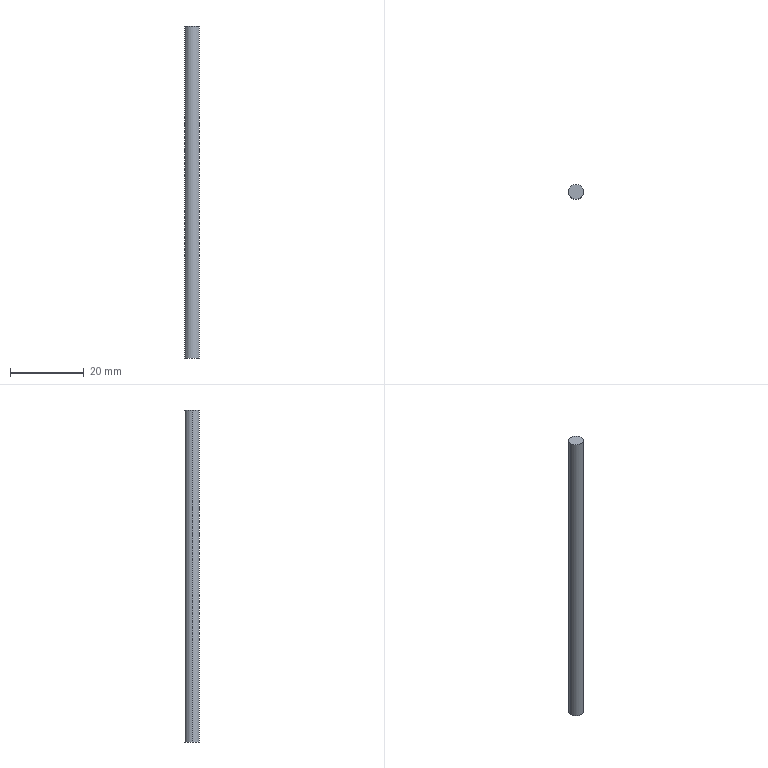Part | SolidWorks | features Extrusion 1 | 1 solid | 4 faces | box 4 x 4 x 90 mm | volume 1131 mm3 | cylinder 2 | plane 2 | commonest cylinder face diameters 4 x2
STEP:
#1=CARTESIAN_POINT('',(2.,0.,90.));
#2=VERTEX_POINT('',#1);
#3=CARTESIAN_POINT('',(-2.,0.,90.));
#4=VERTEX_POINT('',#3);
#5=CARTESIAN_POINT('',(0.,0.,90.));
#6=DIRECTION('',(0.,0.,1.));
#7=DIRECTION('',(1.,0.,0.));
#8=AXIS2_PLACEMENT_3D('',#5,#6,#7);
#9=CIRCLE('',#8,2.);
#10=EDGE_CURVE('',#2,#4,#9,.T.);
#11=ORIENTED_EDGE('',*,*,#10,.F.);
#12=CARTESIAN_POINT('',(2.,0.,0.));
#13=VERTEX_POINT('',#12);
#14=CARTESIAN_POINT('',(2.,0.,90.));
#15=DIRECTION('',(0.,0.,-1.));
#16=VECTOR('',#15,1000.);
#17=LINE('',#14,#16);
#18=EDGE_CURVE('',#2,#13,#17,.T.);
#19=ORIENTED_EDGE('',*,*,#18,.T.);
#20=CARTESIAN_POINT('',(-2.,0.,0.));
#21=VERTEX_POINT('',#20);
#22=CARTESIAN_POINT('',(0.,0.,0.));
#23=DIRECTION('',(0.,0.,1.));
#24=DIRECTION('',(1.,0.,0.));
#25=AXIS2_PLACEMENT_3D('',#22,#23,#24);
#26=CIRCLE('',#25,2.);
#27=EDGE_CURVE('',#13,#21,#26,.T.);
#28=ORIENTED_EDGE('',*,*,#27,.T.);
#29=CARTESIAN_POINT('',(-2.,0.,90.));
#30=DIRECTION('',(0.,0.,-1.));
#31=VECTOR('',#30,1000.);
#32=LINE('',#29,#31);
#33=EDGE_CURVE('',#4,#21,#32,.T.);
#34=ORIENTED_EDGE('',*,*,#33,.F.);
#35=EDGE_LOOP('',(#11,#19,#28,#34));
#36=FACE_OUTER_BOUND('',#35,.T.);
#37=CARTESIAN_POINT('',(0.,0.,90.));
#38=DIRECTION('',(0.,0.,-1.));
#39=DIRECTION('',(-1.,0.,0.));
#40=AXIS2_PLACEMENT_3D('',#37,#38,#39);
#41=CYLINDRICAL_SURFACE('',#40,2.);
#42=ADVANCED_FACE('',(#36),#41,.T.);
#43=ORIENTED_EDGE('',*,*,#18,.F.);
#44=CARTESIAN_POINT('',(0.,0.,90.));
#45=DIRECTION('',(0.,0.,1.));
#46=DIRECTION('',(1.,0.,0.));
#47=AXIS2_PLACEMENT_3D('',#44,#45,#46);
#48=CIRCLE('',#47,2.);
#49=EDGE_CURVE('',#4,#2,#48,.T.);
#50=ORIENTED_EDGE('',*,*,#49,.F.);
#51=ORIENTED_EDGE('',*,*,#33,.T.);
#52=CARTESIAN_POINT('',(0.,0.,0.));
#53=DIRECTION('',(0.,0.,1.));
#54=DIRECTION('',(1.,0.,0.));
#55=AXIS2_PLACEMENT_3D('',#52,#53,#54);
#56=CIRCLE('',#55,2.);
#57=EDGE_CURVE('',#21,#13,#56,.T.);
#58=ORIENTED_EDGE('',*,*,#57,.T.);
#59=EDGE_LOOP('',(#43,#50,#51,#58));
#60=FACE_OUTER_BOUND('',#59,.T.);
#61=CARTESIAN_POINT('',(0.,0.,90.));
#62=DIRECTION('',(0.,0.,-1.));
#63=DIRECTION('',(-1.,0.,0.));
#64=AXIS2_PLACEMENT_3D('',#61,#62,#63);
#65=CYLINDRICAL_SURFACE('',#64,2.);
#66=ADVANCED_FACE('',(#60),#65,.T.);
#67=ORIENTED_EDGE('',*,*,#49,.T.);
#68=ORIENTED_EDGE('',*,*,#10,.T.);
#69=EDGE_LOOP('',(#67,#68));
#70=FACE_OUTER_BOUND('',#69,.T.);
#71=CARTESIAN_POINT('',(0.,0.,90.));
#72=DIRECTION('',(0.,0.,1.));
#73=DIRECTION('',(1.,0.,0.));
#74=AXIS2_PLACEMENT_3D('',#71,#72,#73);
#75=PLANE('',#74);
#76=ADVANCED_FACE('',(#70),#75,.T.);
#77=ORIENTED_EDGE('',*,*,#57,.F.);
#78=ORIENTED_EDGE('',*,*,#27,.F.);
#79=EDGE_LOOP('',(#77,#78));
#80=FACE_OUTER_BOUND('',#79,.T.);
#81=CARTESIAN_POINT('',(0.,0.,0.));
#82=DIRECTION('',(0.,0.,1.));
#83=DIRECTION('',(1.,0.,0.));
#84=AXIS2_PLACEMENT_3D('',#81,#82,#83);
#85=PLANE('',#84);
#86=ADVANCED_FACE('',(#80),#85,.F.);
#87=CLOSED_SHELL('',(#42,#66,#76,#86));
#88=MANIFOLD_SOLID_BREP('',#87);
#89=CARTESIAN_POINT('',(0.,0.,0.));
#90=DIRECTION('',(0.,0.,1.));
#91=DIRECTION('',(1.,0.,0.));
#92=AXIS2_PLACEMENT_3D('',#89,#90,#91);
#93=(LENGTH_UNIT()NAMED_UNIT(*)SI_UNIT(.MILLI.,.METRE.));
#94=UNCERTAINTY_MEASURE_WITH_UNIT(LENGTH_MEASURE(0.00001),#93,'','');
#95=(NAMED_UNIT(*)PLANE_ANGLE_UNIT()SI_UNIT($,.RADIAN.));
#96=(NAMED_UNIT(*)SI_UNIT($,.STERADIAN.)SOLID_ANGLE_UNIT());
#97=(GEOMETRIC_REPRESENTATION_CONTEXT(3)GLOBAL_UNCERTAINTY_ASSIGNED_CONTEXT((#94))GLOBAL_UNIT_ASSIGNED_CONTEXT((#93,#95,#96))REPRESENTATION_CONTEXT('',''));
#98=ADVANCED_BREP_SHAPE_REPRESENTATION('',(#88,#92),#97);